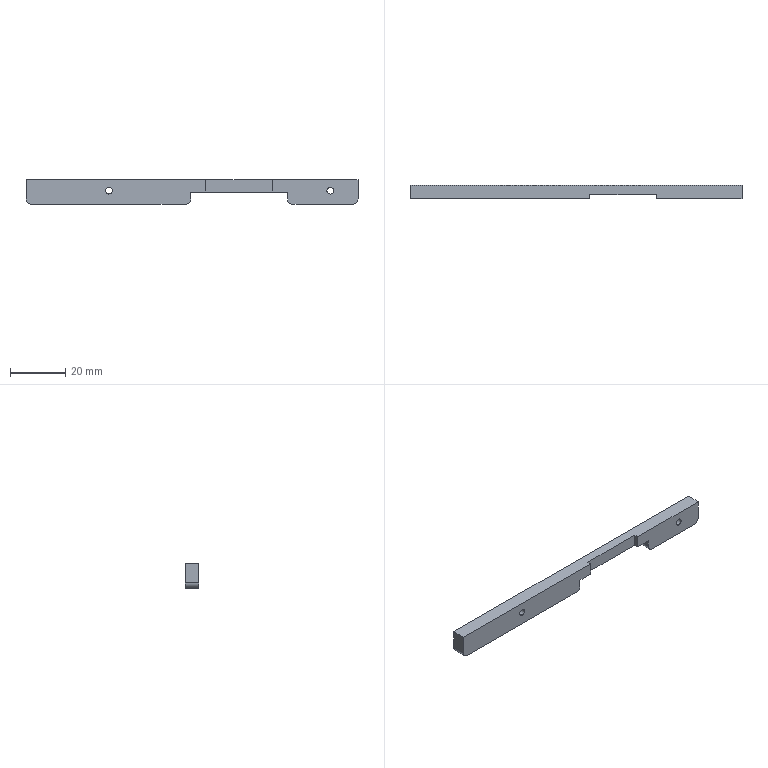Part | SolidWorks | features Fillet 2, ICE 2, Extrusion 1, HoleWzd 1 | 1 solid | 22 faces | box 120 x 5 x 9 mm | volume 4384 mm3 | plane 14 | cylinder 8 | commonest cylinder face diameters 2.5 x4 4 x4
STEP:
#1=CARTESIAN_POINT('',(30.,0.,-2.75));
#2=VERTEX_POINT('',#1);
#3=CARTESIAN_POINT('',(30.,0.,-5.25));
#4=VERTEX_POINT('',#3);
#5=CARTESIAN_POINT('',(30.,0.,-4.));
#6=DIRECTION('',(0.,-1.,0.));
#7=DIRECTION('',(0.,0.,-1.));
#8=AXIS2_PLACEMENT_3D('',#5,#6,#7);
#9=CIRCLE('',#8,1.25);
#10=EDGE_CURVE('',#2,#4,#9,.T.);
#11=ORIENTED_EDGE('',*,*,#10,.T.);
#12=CARTESIAN_POINT('',(30.,5.,-5.25));
#13=VERTEX_POINT('',#12);
#14=CARTESIAN_POINT('',(30.,5.,-5.25));
#15=DIRECTION('',(0.,1.,0.));
#16=VECTOR('',#15,1000.);
#17=LINE('',#14,#16);
#18=EDGE_CURVE('',#4,#13,#17,.T.);
#19=ORIENTED_EDGE('',*,*,#18,.T.);
#20=CARTESIAN_POINT('',(30.,5.,-2.75));
#21=VERTEX_POINT('',#20);
#22=CARTESIAN_POINT('',(30.,5.,-4.));
#23=DIRECTION('',(0.,1.,0.));
#24=DIRECTION('',(0.,0.,1.));
#25=AXIS2_PLACEMENT_3D('',#22,#23,#24);
#26=CIRCLE('',#25,1.25);
#27=EDGE_CURVE('',#13,#21,#26,.T.);
#28=ORIENTED_EDGE('',*,*,#27,.T.);
#29=CARTESIAN_POINT('',(30.,5.,-2.75));
#30=DIRECTION('',(0.,1.,0.));
#31=VECTOR('',#30,1000.);
#32=LINE('',#29,#31);
#33=EDGE_CURVE('',#2,#21,#32,.T.);
#34=ORIENTED_EDGE('',*,*,#33,.F.);
#35=EDGE_LOOP('',(#11,#19,#28,#34));
#36=FACE_OUTER_BOUND('',#35,.T.);
#37=CARTESIAN_POINT('',(30.,5.,-4.));
#38=DIRECTION('',(0.,1.,0.));
#39=DIRECTION('',(0.,0.,1.));
#40=AXIS2_PLACEMENT_3D('',#37,#38,#39);
#41=CYLINDRICAL_SURFACE('',#40,1.25);
#42=ADVANCED_FACE('',(#36),#41,.F.);
#43=CARTESIAN_POINT('',(110.,0.,-2.75));
#44=VERTEX_POINT('',#43);
#45=CARTESIAN_POINT('',(110.,0.,-5.25));
#46=VERTEX_POINT('',#45);
#47=CARTESIAN_POINT('',(110.,0.,-4.));
#48=DIRECTION('',(0.,-1.,0.));
#49=DIRECTION('',(0.,0.,-1.));
#50=AXIS2_PLACEMENT_3D('',#47,#48,#49);
#51=CIRCLE('',#50,1.25);
#52=EDGE_CURVE('',#44,#46,#51,.T.);
#53=ORIENTED_EDGE('',*,*,#52,.T.);
#54=CARTESIAN_POINT('',(110.,5.,-5.25));
#55=VERTEX_POINT('',#54);
#56=CARTESIAN_POINT('',(110.,5.,-5.25));
#57=DIRECTION('',(0.,1.,0.));
#58=VECTOR('',#57,1000.);
#59=LINE('',#56,#58);
#60=EDGE_CURVE('',#46,#55,#59,.T.);
#61=ORIENTED_EDGE('',*,*,#60,.T.);
#62=CARTESIAN_POINT('',(110.,5.,-2.75));
#63=VERTEX_POINT('',#62);
#64=CARTESIAN_POINT('',(110.,5.,-4.));
#65=DIRECTION('',(0.,1.,0.));
#66=DIRECTION('',(0.,0.,1.));
#67=AXIS2_PLACEMENT_3D('',#64,#65,#66);
#68=CIRCLE('',#67,1.25);
#69=EDGE_CURVE('',#55,#63,#68,.T.);
#70=ORIENTED_EDGE('',*,*,#69,.T.);
#71=CARTESIAN_POINT('',(110.,5.,-2.75));
#72=DIRECTION('',(0.,1.,0.));
#73=VECTOR('',#72,1000.);
#74=LINE('',#71,#73);
#75=EDGE_CURVE('',#44,#63,#74,.T.);
#76=ORIENTED_EDGE('',*,*,#75,.F.);
#77=EDGE_LOOP('',(#53,#61,#70,#76));
#78=FACE_OUTER_BOUND('',#77,.T.);
#79=CARTESIAN_POINT('',(110.,5.,-4.));
#80=DIRECTION('',(0.,1.,0.));
#81=DIRECTION('',(0.,0.,1.));
#82=AXIS2_PLACEMENT_3D('',#79,#80,#81);
#83=CYLINDRICAL_SURFACE('',#82,1.25);
#84=ADVANCED_FACE('',(#78),#83,.F.);
#85=CARTESIAN_POINT('',(65.,0.,0.));
#86=VERTEX_POINT('',#85);
#87=CARTESIAN_POINT('',(65.,0.,-4.5));
#88=VERTEX_POINT('',#87);
#89=CARTESIAN_POINT('',(65.,0.,-9.));
#90=DIRECTION('',(0.,0.,-1.));
#91=VECTOR('',#90,1000.);
#92=LINE('',#89,#91);
#93=EDGE_CURVE('',#86,#88,#92,.T.);
#94=ORIENTED_EDGE('',*,*,#93,.F.);
#95=CARTESIAN_POINT('',(0.,0.,0.));
#96=VERTEX_POINT('',#95);
#97=CARTESIAN_POINT('',(120.,0.,0.));
#98=DIRECTION('',(1.,0.,0.));
#99=VECTOR('',#98,1000.);
#100=LINE('',#97,#99);
#101=EDGE_CURVE('',#96,#86,#100,.T.);
#102=ORIENTED_EDGE('',*,*,#101,.F.);
#103=CARTESIAN_POINT('',(0.,0.,-7.));
#104=VERTEX_POINT('',#103);
#105=CARTESIAN_POINT('',(0.,0.,0.));
#106=DIRECTION('',(0.,0.,1.));
#107=VECTOR('',#106,1000.);
#108=LINE('',#105,#107);
#109=EDGE_CURVE('',#104,#96,#108,.T.);
#110=ORIENTED_EDGE('',*,*,#109,.F.);
#111=CARTESIAN_POINT('',(2.,0.,-9.));
#112=VERTEX_POINT('',#111);
#113=CARTESIAN_POINT('',(2.,0.,-7.));
#114=DIRECTION('',(0.,-1.,0.));
#115=DIRECTION('',(0.,0.,-1.));
#116=AXIS2_PLACEMENT_3D('',#113,#114,#115);
#117=CIRCLE('',#116,2.);
#118=EDGE_CURVE('',#104,#112,#117,.T.);
#119=ORIENTED_EDGE('',*,*,#118,.T.);
#120=CARTESIAN_POINT('',(57.5,0.,-9.));
#121=VERTEX_POINT('',#120);
#122=CARTESIAN_POINT('',(0.,0.,-9.));
#123=DIRECTION('',(-1.,0.,0.));
#124=VECTOR('',#123,1000.);
#125=LINE('',#122,#124);
#126=EDGE_CURVE('',#121,#112,#125,.T.);
#127=ORIENTED_EDGE('',*,*,#126,.F.);
#128=CARTESIAN_POINT('',(59.5,0.,-7.));
#129=VERTEX_POINT('',#128);
#130=CARTESIAN_POINT('',(57.5,0.,-7.));
#131=DIRECTION('',(0.,-1.,0.));
#132=DIRECTION('',(0.,0.,-1.));
#133=AXIS2_PLACEMENT_3D('',#130,#131,#132);
#134=CIRCLE('',#133,2.);
#135=EDGE_CURVE('',#121,#129,#134,.T.);
#136=ORIENTED_EDGE('',*,*,#135,.T.);
#137=CARTESIAN_POINT('',(59.5,0.,-4.5));
#138=VERTEX_POINT('',#137);
#139=CARTESIAN_POINT('',(59.5,0.,-9.));
#140=DIRECTION('',(0.,0.,1.));
#141=VECTOR('',#140,1000.);
#142=LINE('',#139,#141);
#143=EDGE_CURVE('',#129,#138,#142,.T.);
#144=ORIENTED_EDGE('',*,*,#143,.T.);
#145=CARTESIAN_POINT('',(94.5,0.,-4.5));
#146=DIRECTION('',(1.,0.,0.));
#147=VECTOR('',#146,1000.);
#148=LINE('',#145,#147);
#149=EDGE_CURVE('',#138,#88,#148,.T.);
#150=ORIENTED_EDGE('',*,*,#149,.T.);
#151=EDGE_LOOP('',(#94,#102,#110,#119,#127,#136,#144,#150));
#152=FACE_OUTER_BOUND('',#151,.T.);
#153=ORIENTED_EDGE('',*,*,#10,.F.);
#154=CARTESIAN_POINT('',(30.,0.,-4.));
#155=DIRECTION('',(0.,-1.,0.));
#156=DIRECTION('',(0.,0.,-1.));
#157=AXIS2_PLACEMENT_3D('',#154,#155,#156);
#158=CIRCLE('',#157,1.25);
#159=EDGE_CURVE('',#4,#2,#158,.T.);
#160=ORIENTED_EDGE('',*,*,#159,.F.);
#161=EDGE_LOOP('',(#153,#160));
#162=FACE_BOUND('',#161,.T.);
#163=CARTESIAN_POINT('',(0.,0.,0.));
#164=DIRECTION('',(0.,-1.,0.));
#165=DIRECTION('',(0.,0.,-1.));
#166=AXIS2_PLACEMENT_3D('',#163,#164,#165);
#167=PLANE('',#166);
#168=ADVANCED_FACE('',(#152,#162),#167,.T.);
#169=CARTESIAN_POINT('',(118.,0.,-9.));
#170=VERTEX_POINT('',#169);
#171=CARTESIAN_POINT('',(96.5,0.,-9.));
#172=VERTEX_POINT('',#171);
#173=CARTESIAN_POINT('',(0.,0.,-9.));
#174=DIRECTION('',(-1.,0.,0.));
#175=VECTOR('',#174,1000.);
#176=LINE('',#173,#175);
#177=EDGE_CURVE('',#170,#172,#176,.T.);
#178=ORIENTED_EDGE('',*,*,#177,.T.);
#179=CARTESIAN_POINT('',(96.5,5.,-9.));
#180=VERTEX_POINT('',#179);
#181=CARTESIAN_POINT('',(96.5,5.,-9.));
#182=DIRECTION('',(0.,1.,0.));
#183=VECTOR('',#182,1000.);
#184=LINE('',#181,#183);
#185=EDGE_CURVE('',#172,#180,#184,.T.);
#186=ORIENTED_EDGE('',*,*,#185,.T.);
#187=CARTESIAN_POINT('',(118.,5.,-9.));
#188=VERTEX_POINT('',#187);
#189=CARTESIAN_POINT('',(0.,5.,-9.));
#190=DIRECTION('',(-1.,0.,0.));
#191=VECTOR('',#190,1000.);
#192=LINE('',#189,#191);
#193=EDGE_CURVE('',#188,#180,#192,.T.);
#194=ORIENTED_EDGE('',*,*,#193,.F.);
#195=CARTESIAN_POINT('',(118.,5.,-9.));
#196=DIRECTION('',(0.,-1.,0.));
#197=VECTOR('',#196,1000.);
#198=LINE('',#195,#197);
#199=EDGE_CURVE('',#188,#170,#198,.T.);
#200=ORIENTED_EDGE('',*,*,#199,.T.);
#201=EDGE_LOOP('',(#178,#186,#194,#200));
#202=FACE_OUTER_BOUND('',#201,.T.);
#203=CARTESIAN_POINT('',(0.,5.,-9.));
#204=DIRECTION('',(0.,0.,1.));
#205=DIRECTION('',(1.,0.,0.));
#206=AXIS2_PLACEMENT_3D('',#203,#204,#205);
#207=PLANE('',#206);
#208=ADVANCED_FACE('',(#202),#207,.F.);
#209=ORIENTED_EDGE('',*,*,#101,.T.);
#210=CARTESIAN_POINT('',(65.,1.5,0.));
#211=VERTEX_POINT('',#210);
#212=CARTESIAN_POINT('',(65.,1.5,0.));
#213=DIRECTION('',(0.,-1.,0.));
#214=VECTOR('',#213,1000.);
#215=LINE('',#212,#214);
#216=EDGE_CURVE('',#211,#86,#215,.T.);
#217=ORIENTED_EDGE('',*,*,#216,.F.);
#218=CARTESIAN_POINT('',(89.,1.5,0.));
#219=VERTEX_POINT('',#218);
#220=CARTESIAN_POINT('',(89.,1.5,0.));
#221=DIRECTION('',(-1.,0.,0.));
#222=VECTOR('',#221,1000.);
#223=LINE('',#220,#222);
#224=EDGE_CURVE('',#219,#211,#223,.T.);
#225=ORIENTED_EDGE('',*,*,#224,.F.);
#226=CARTESIAN_POINT('',(89.,0.,0.));
#227=VERTEX_POINT('',#226);
#228=CARTESIAN_POINT('',(89.,1.5,0.));
#229=DIRECTION('',(0.,-1.,0.));
#230=VECTOR('',#229,1000.);
#231=LINE('',#228,#230);
#232=EDGE_CURVE('',#219,#227,#231,.T.);
#233=ORIENTED_EDGE('',*,*,#232,.T.);
#234=CARTESIAN_POINT('',(120.,0.,0.));
#235=VERTEX_POINT('',#234);
#236=CARTESIAN_POINT('',(120.,0.,0.));
#237=DIRECTION('',(1.,0.,0.));
#238=VECTOR('',#237,1000.);
#239=LINE('',#236,#238);
#240=EDGE_CURVE('',#227,#235,#239,.T.);
#241=ORIENTED_EDGE('',*,*,#240,.T.);
#242=CARTESIAN_POINT('',(120.,5.,0.));
#243=VERTEX_POINT('',#242);
#244=CARTESIAN_POINT('',(120.,5.,0.));
#245=DIRECTION('',(0.,-1.,0.));
#246=VECTOR('',#245,1000.);
#247=LINE('',#244,#246);
#248=EDGE_CURVE('',#243,#235,#247,.T.);
#249=ORIENTED_EDGE('',*,*,#248,.F.);
#250=CARTESIAN_POINT('',(0.,5.,0.));
#251=VERTEX_POINT('',#250);
#252=CARTESIAN_POINT('',(120.,5.,0.));
#253=DIRECTION('',(1.,0.,0.));
#254=VECTOR('',#253,1000.);
#255=LINE('',#252,#254);
#256=EDGE_CURVE('',#251,#243,#255,.T.);
#257=ORIENTED_EDGE('',*,*,#256,.F.);
#258=CARTESIAN_POINT('',(0.,5.,0.));
#259=DIRECTION('',(0.,-1.,0.));
#260=VECTOR('',#259,1000.);
#261=LINE('',#258,#260);
#262=EDGE_CURVE('',#251,#96,#261,.T.);
#263=ORIENTED_EDGE('',*,*,#262,.T.);
#264=EDGE_LOOP('',(#209,#217,#225,#233,#241,#249,#257,#263));
#265=FACE_OUTER_BOUND('',#264,.T.);
#266=CARTESIAN_POINT('',(120.,5.,0.));
#267=DIRECTION('',(0.,0.,-1.));
#268=DIRECTION('',(-1.,0.,0.));
#269=AXIS2_PLACEMENT_3D('',#266,#267,#268);
#270=PLANE('',#269);
#271=ADVANCED_FACE('',(#265),#270,.F.);
#272=CARTESIAN_POINT('',(120.,0.,-7.));
#273=VERTEX_POINT('',#272);
#274=CARTESIAN_POINT('',(120.,0.,-9.));
#275=DIRECTION('',(0.,0.,-1.));
#276=VECTOR('',#275,1000.);
#277=LINE('',#274,#276);
#278=EDGE_CURVE('',#235,#273,#277,.T.);
#279=ORIENTED_EDGE('',*,*,#278,.T.);
#280=CARTESIAN_POINT('',(120.,5.,-7.));
#281=VERTEX_POINT('',#280);
#282=CARTESIAN_POINT('',(120.,5.,-7.));
#283=DIRECTION('',(0.,1.,0.));
#284=VECTOR('',#283,1000.);
#285=LINE('',#282,#284);
#286=EDGE_CURVE('',#273,#281,#285,.T.);
#287=ORIENTED_EDGE('',*,*,#286,.T.);
#288=CARTESIAN_POINT('',(120.,5.,-9.));
#289=DIRECTION('',(0.,0.,-1.));
#290=VECTOR('',#289,1000.);
#291=LINE('',#288,#290);
#292=EDGE_CURVE('',#243,#281,#291,.T.);
#293=ORIENTED_EDGE('',*,*,#292,.F.);
#294=ORIENTED_EDGE('',*,*,#248,.T.);
#295=EDGE_LOOP('',(#279,#287,#293,#294));
#296=FACE_OUTER_BOUND('',#295,.T.);
#297=CARTESIAN_POINT('',(120.,5.,-9.));
#298=DIRECTION('',(-1.,0.,0.));
#299=DIRECTION('',(0.,0.,1.));
#300=AXIS2_PLACEMENT_3D('',#297,#298,#299);
#301=PLANE('',#300);
#302=ADVANCED_FACE('',(#296),#301,.F.);
#303=CARTESIAN_POINT('',(57.5,5.,-9.));
#304=VERTEX_POINT('',#303);
#305=CARTESIAN_POINT('',(2.,5.,-9.));
#306=VERTEX_POINT('',#305);
#307=CARTESIAN_POINT('',(0.,5.,-9.));
#308=DIRECTION('',(-1.,0.,0.));
#309=VECTOR('',#308,1000.);
#310=LINE('',#307,#309);
#311=EDGE_CURVE('',#304,#306,#310,.T.);
#312=ORIENTED_EDGE('',*,*,#311,.F.);
#313=CARTESIAN_POINT('',(57.5,5.,-9.));
#314=DIRECTION('',(0.,-1.,0.));
#315=VECTOR('',#314,1000.);
#316=LINE('',#313,#315);
#317=EDGE_CURVE('',#304,#121,#316,.T.);
#318=ORIENTED_EDGE('',*,*,#317,.T.);
#319=ORIENTED_EDGE('',*,*,#126,.T.);
#320=CARTESIAN_POINT('',(2.,5.,-9.));
#321=DIRECTION('',(0.,1.,0.));
#322=VECTOR('',#321,1000.);
#323=LINE('',#320,#322);
#324=EDGE_CURVE('',#112,#306,#323,.T.);
#325=ORIENTED_EDGE('',*,*,#324,.T.);
#326=EDGE_LOOP('',(#312,#318,#319,#325));
#327=FACE_OUTER_BOUND('',#326,.T.);
#328=CARTESIAN_POINT('',(0.,5.,-9.));
#329=DIRECTION('',(0.,0.,1.));
#330=DIRECTION('',(1.,0.,0.));
#331=AXIS2_PLACEMENT_3D('',#328,#329,#330);
#332=PLANE('',#331);
#333=ADVANCED_FACE('',(#327),#332,.F.);
#334=CARTESIAN_POINT('',(0.,5.,-7.));
#335=VERTEX_POINT('',#334);
#336=CARTESIAN_POINT('',(0.,5.,0.));
#337=DIRECTION('',(0.,0.,1.));
#338=VECTOR('',#337,1000.);
#339=LINE('',#336,#338);
#340=EDGE_CURVE('',#335,#251,#339,.T.);
#341=ORIENTED_EDGE('',*,*,#340,.F.);
#342=CARTESIAN_POINT('',(0.,5.,-7.));
#343=DIRECTION('',(0.,-1.,0.));
#344=VECTOR('',#343,1000.);
#345=LINE('',#342,#344);
#346=EDGE_CURVE('',#335,#104,#345,.T.);
#347=ORIENTED_EDGE('',*,*,#346,.T.);
#348=ORIENTED_EDGE('',*,*,#109,.T.);
#349=ORIENTED_EDGE('',*,*,#262,.F.);
#350=EDGE_LOOP('',(#341,#347,#348,#349));
#351=FACE_OUTER_BOUND('',#350,.T.);
#352=CARTESIAN_POINT('',(0.,5.,0.));
#353=DIRECTION('',(1.,0.,0.));
#354=DIRECTION('',(0.,0.,-1.));
#355=AXIS2_PLACEMENT_3D('',#352,#353,#354);
#356=PLANE('',#355);
#357=ADVANCED_FACE('',(#351),#356,.F.);
#358=CARTESIAN_POINT('',(30.,5.,-4.));
#359=DIRECTION('',(0.,1.,0.));
#360=DIRECTION('',(0.,0.,1.));
#361=AXIS2_PLACEMENT_3D('',#358,#359,#360);
#362=CIRCLE('',#361,1.25);
#363=EDGE_CURVE('',#21,#13,#362,.T.);
#364=ORIENTED_EDGE('',*,*,#363,.F.);
#365=ORIENTED_EDGE('',*,*,#27,.F.);
#366=EDGE_LOOP('',(#364,#365));
#367=FACE_BOUND('',#366,.T.);
#368=CARTESIAN_POINT('',(110.,5.,-4.));
#369=DIRECTION('',(0.,1.,0.));
#370=DIRECTION('',(0.,0.,1.));
#371=AXIS2_PLACEMENT_3D('',#368,#369,#370);
#372=CIRCLE('',#371,1.25);
#373=EDGE_CURVE('',#63,#55,#372,.T.);
#374=ORIENTED_EDGE('',*,*,#373,.F.);
#375=ORIENTED_EDGE('',*,*,#69,.F.);
#376=EDGE_LOOP('',(#374,#375));
#377=FACE_BOUND('',#376,.T.);
#378=ORIENTED_EDGE('',*,*,#193,.T.);
#379=CARTESIAN_POINT('',(94.5,5.,-7.));
#380=VERTEX_POINT('',#379);
#381=CARTESIAN_POINT('',(96.5,5.,-7.));
#382=DIRECTION('',(0.,1.,0.));
#383=DIRECTION('',(0.,0.,-1.));
#384=AXIS2_PLACEMENT_3D('',#381,#382,#383);
#385=CIRCLE('',#384,2.);
#386=EDGE_CURVE('',#180,#380,#385,.T.);
#387=ORIENTED_EDGE('',*,*,#386,.T.);
#388=CARTESIAN_POINT('',(94.5,5.,-4.5));
#389=VERTEX_POINT('',#388);
#390=CARTESIAN_POINT('',(94.5,5.,-9.));
#391=DIRECTION('',(0.,0.,-1.));
#392=VECTOR('',#391,1000.);
#393=LINE('',#390,#392);
#394=EDGE_CURVE('',#389,#380,#393,.T.);
#395=ORIENTED_EDGE('',*,*,#394,.F.);
#396=CARTESIAN_POINT('',(59.5,5.,-4.5));
#397=VERTEX_POINT('',#396);
#398=CARTESIAN_POINT('',(94.5,5.,-4.5));
#399=DIRECTION('',(1.,0.,0.));
#400=VECTOR('',#399,1000.);
#401=LINE('',#398,#400);
#402=EDGE_CURVE('',#397,#389,#401,.T.);
#403=ORIENTED_EDGE('',*,*,#402,.F.);
#404=CARTESIAN_POINT('',(59.5,5.,-7.));
#405=VERTEX_POINT('',#404);
#406=CARTESIAN_POINT('',(59.5,5.,-9.));
#407=DIRECTION('',(0.,0.,1.));
#408=VECTOR('',#407,1000.);
#409=LINE('',#406,#408);
#410=EDGE_CURVE('',#405,#397,#409,.T.);
#411=ORIENTED_EDGE('',*,*,#410,.F.);
#412=CARTESIAN_POINT('',(57.5,5.,-7.));
#413=DIRECTION('',(0.,1.,0.));
#414=DIRECTION('',(0.,0.,-1.));
#415=AXIS2_PLACEMENT_3D('',#412,#413,#414);
#416=CIRCLE('',#415,2.);
#417=EDGE_CURVE('',#405,#304,#416,.T.);
#418=ORIENTED_EDGE('',*,*,#417,.T.);
#419=ORIENTED_EDGE('',*,*,#311,.T.);
#420=CARTESIAN_POINT('',(2.,5.,-7.));
#421=DIRECTION('',(0.,1.,0.));
#422=DIRECTION('',(0.,0.,-1.));
#423=AXIS2_PLACEMENT_3D('',#420,#421,#422);
#424=CIRCLE('',#423,2.);
#425=EDGE_CURVE('',#306,#335,#424,.T.);
#426=ORIENTED_EDGE('',*,*,#425,.T.);
#427=ORIENTED_EDGE('',*,*,#340,.T.);
#428=ORIENTED_EDGE('',*,*,#256,.T.);
#429=ORIENTED_EDGE('',*,*,#292,.T.);
#430=CARTESIAN_POINT('',(118.,5.,-7.));
#431=DIRECTION('',(0.,1.,0.));
#432=DIRECTION('',(0.,0.,-1.));
#433=AXIS2_PLACEMENT_3D('',#430,#431,#432);
#434=CIRCLE('',#433,2.);
#435=EDGE_CURVE('',#281,#188,#434,.T.);
#436=ORIENTED_EDGE('',*,*,#435,.T.);
#437=EDGE_LOOP('',(#378,#387,#395,#403,#411,#418,#419,#426,#427,#428,#429,#436));
#438=FACE_OUTER_BOUND('',#437,.T.);
#439=CARTESIAN_POINT('',(0.,5.,0.));
#440=DIRECTION('',(0.,-1.,0.));
#441=DIRECTION('',(0.,0.,-1.));
#442=AXIS2_PLACEMENT_3D('',#439,#440,#441);
#443=PLANE('',#442);
#444=ADVANCED_FACE('',(#367,#377,#438),#443,.F.);
#445=CARTESIAN_POINT('',(89.,0.,-4.5));
#446=VERTEX_POINT('',#445);
#447=CARTESIAN_POINT('',(89.,0.,-9.));
#448=DIRECTION('',(0.,0.,1.));
#449=VECTOR('',#448,1000.);
#450=LINE('',#447,#449);
#451=EDGE_CURVE('',#446,#227,#450,.T.);
#452=ORIENTED_EDGE('',*,*,#451,.F.);
#453=CARTESIAN_POINT('',(94.5,0.,-4.5));
#454=VERTEX_POINT('',#453);
#455=CARTESIAN_POINT('',(94.5,0.,-4.5));
#456=DIRECTION('',(1.,0.,0.));
#457=VECTOR('',#456,1000.);
#458=LINE('',#455,#457);
#459=EDGE_CURVE('',#446,#454,#458,.T.);
#460=ORIENTED_EDGE('',*,*,#459,.T.);
#461=CARTESIAN_POINT('',(94.5,0.,-7.));
#462=VERTEX_POINT('',#461);
#463=CARTESIAN_POINT('',(94.5,0.,-9.));
#464=DIRECTION('',(0.,0.,-1.));
#465=VECTOR('',#464,1000.);
#466=LINE('',#463,#465);
#467=EDGE_CURVE('',#454,#462,#466,.T.);
#468=ORIENTED_EDGE('',*,*,#467,.T.);
#469=CARTESIAN_POINT('',(96.5,0.,-7.));
#470=DIRECTION('',(0.,-1.,0.));
#471=DIRECTION('',(0.,0.,-1.));
#472=AXIS2_PLACEMENT_3D('',#469,#470,#471);
#473=CIRCLE('',#472,2.);
#474=EDGE_CURVE('',#462,#172,#473,.T.);
#475=ORIENTED_EDGE('',*,*,#474,.T.);
#476=ORIENTED_EDGE('',*,*,#177,.F.);
#477=CARTESIAN_POINT('',(118.,0.,-7.));
#478=DIRECTION('',(0.,-1.,0.));
#479=DIRECTION('',(0.,0.,-1.));
#480=AXIS2_PLACEMENT_3D('',#477,#478,#479);
#481=CIRCLE('',#480,2.);
#482=EDGE_CURVE('',#170,#273,#481,.T.);
#483=ORIENTED_EDGE('',*,*,#482,.T.);
#484=ORIENTED_EDGE('',*,*,#278,.F.);
#485=ORIENTED_EDGE('',*,*,#240,.F.);
#486=EDGE_LOOP('',(#452,#460,#468,#475,#476,#483,#484,#485));
#487=FACE_OUTER_BOUND('',#486,.T.);
#488=ORIENTED_EDGE('',*,*,#52,.F.);
#489=CARTESIAN_POINT('',(110.,0.,-4.));
#490=DIRECTION('',(0.,-1.,0.));
#491=DIRECTION('',(0.,0.,-1.));
#492=AXIS2_PLACEMENT_3D('',#489,#490,#491);
#493=CIRCLE('',#492,1.25);
#494=EDGE_CURVE('',#46,#44,#493,.T.);
#495=ORIENTED_EDGE('',*,*,#494,.F.);
#496=EDGE_LOOP('',(#488,#495));
#497=FACE_BOUND('',#496,.T.);
#498=CARTESIAN_POINT('',(0.,0.,0.));
#499=DIRECTION('',(0.,-1.,0.));
#500=DIRECTION('',(0.,0.,-1.));
#501=AXIS2_PLACEMENT_3D('',#498,#499,#500);
#502=PLANE('',#501);
#503=ADVANCED_FACE('',(#487,#497),#502,.T.);
#504=ORIENTED_EDGE('',*,*,#60,.F.);
#505=ORIENTED_EDGE('',*,*,#494,.T.);
#506=ORIENTED_EDGE('',*,*,#75,.T.);
#507=ORIENTED_EDGE('',*,*,#373,.T.);
#508=EDGE_LOOP('',(#504,#505,#506,#507));
#509=FACE_OUTER_BOUND('',#508,.T.);
#510=CARTESIAN_POINT('',(110.,5.,-4.));
#511=DIRECTION('',(0.,1.,0.));
#512=DIRECTION('',(0.,0.,1.));
#513=AXIS2_PLACEMENT_3D('',#510,#511,#512);
#514=CYLINDRICAL_SURFACE('',#513,1.25);
#515=ADVANCED_FACE('',(#509),#514,.F.);
#516=ORIENTED_EDGE('',*,*,#18,.F.);
#517=ORIENTED_EDGE('',*,*,#159,.T.);
#518=ORIENTED_EDGE('',*,*,#33,.T.);
#519=ORIENTED_EDGE('',*,*,#363,.T.);
#520=EDGE_LOOP('',(#516,#517,#518,#519));
#521=FACE_OUTER_BOUND('',#520,.T.);
#522=CARTESIAN_POINT('',(30.,5.,-4.));
#523=DIRECTION('',(0.,1.,0.));
#524=DIRECTION('',(0.,0.,1.));
#525=AXIS2_PLACEMENT_3D('',#522,#523,#524);
#526=CYLINDRICAL_SURFACE('',#525,1.25);
#527=ADVANCED_FACE('',(#521),#526,.F.);
#528=ORIENTED_EDGE('',*,*,#425,.F.);
#529=ORIENTED_EDGE('',*,*,#324,.F.);
#530=ORIENTED_EDGE('',*,*,#118,.F.);
#531=ORIENTED_EDGE('',*,*,#346,.F.);
#532=EDGE_LOOP('',(#528,#529,#530,#531));
#533=FACE_OUTER_BOUND('',#532,.T.);
#534=CARTESIAN_POINT('',(2.,5.,-7.));
#535=DIRECTION('',(0.,-1.,0.));
#536=DIRECTION('',(0.,0.,-1.));
#537=AXIS2_PLACEMENT_3D('',#534,#535,#536);
#538=CYLINDRICAL_SURFACE('',#537,2.);
#539=ADVANCED_FACE('',(#533),#538,.T.);
#540=ORIENTED_EDGE('',*,*,#435,.F.);
#541=ORIENTED_EDGE('',*,*,#286,.F.);
#542=ORIENTED_EDGE('',*,*,#482,.F.);
#543=ORIENTED_EDGE('',*,*,#199,.F.);
#544=EDGE_LOOP('',(#540,#541,#542,#543));
#545=FACE_OUTER_BOUND('',#544,.T.);
#546=CARTESIAN_POINT('',(118.,5.,-7.));
#547=DIRECTION('',(0.,-1.,0.));
#548=DIRECTION('',(0.,0.,-1.));
#549=AXIS2_PLACEMENT_3D('',#546,#547,#548);
#550=CYLINDRICAL_SURFACE('',#549,2.);
#551=ADVANCED_FACE('',(#545),#550,.T.);
#552=ORIENTED_EDGE('',*,*,#394,.T.);
#553=CARTESIAN_POINT('',(94.5,0.,-7.));
#554=DIRECTION('',(0.,-1.,0.));
#555=VECTOR('',#554,1000.);
#556=LINE('',#553,#555);
#557=EDGE_CURVE('',#380,#462,#556,.T.);
#558=ORIENTED_EDGE('',*,*,#557,.T.);
#559=ORIENTED_EDGE('',*,*,#467,.F.);
#560=CARTESIAN_POINT('',(94.5,0.,-4.5));
#561=DIRECTION('',(0.,1.,0.));
#562=VECTOR('',#561,1000.);
#563=LINE('',#560,#562);
#564=EDGE_CURVE('',#454,#389,#563,.T.);
#565=ORIENTED_EDGE('',*,*,#564,.T.);
#566=EDGE_LOOP('',(#552,#558,#559,#565));
#567=FACE_OUTER_BOUND('',#566,.T.);
#568=CARTESIAN_POINT('',(94.5,0.,-9.));
#569=DIRECTION('',(1.,0.,0.));
#570=DIRECTION('',(0.,0.,-1.));
#571=AXIS2_PLACEMENT_3D('',#568,#569,#570);
#572=PLANE('',#571);
#573=ADVANCED_FACE('',(#567),#572,.F.);
#574=CARTESIAN_POINT('',(65.,1.5,-4.5));
#575=VERTEX_POINT('',#574);
#576=CARTESIAN_POINT('',(89.,1.5,-4.5));
#577=VERTEX_POINT('',#576);
#578=CARTESIAN_POINT('',(94.5,1.5,-4.5));
#579=DIRECTION('',(1.,0.,0.));
#580=VECTOR('',#579,1000.);
#581=LINE('',#578,#580);
#582=EDGE_CURVE('',#575,#577,#581,.T.);
#583=ORIENTED_EDGE('',*,*,#582,.F.);
#584=CARTESIAN_POINT('',(65.,0.,-4.5));
#585=DIRECTION('',(0.,-1.,0.));
#586=VECTOR('',#585,1000.);
#587=LINE('',#584,#586);
#588=EDGE_CURVE('',#575,#88,#587,.T.);
#589=ORIENTED_EDGE('',*,*,#588,.T.);
#590=ORIENTED_EDGE('',*,*,#149,.F.);
#591=CARTESIAN_POINT('',(59.5,0.,-4.5));
#592=DIRECTION('',(0.,1.,0.));
#593=VECTOR('',#592,1000.);
#594=LINE('',#591,#593);
#595=EDGE_CURVE('',#138,#397,#594,.T.);
#596=ORIENTED_EDGE('',*,*,#595,.T.);
#597=ORIENTED_EDGE('',*,*,#402,.T.);
#598=ORIENTED_EDGE('',*,*,#564,.F.);
#599=ORIENTED_EDGE('',*,*,#459,.F.);
#600=CARTESIAN_POINT('',(89.,0.,-4.5));
#601=DIRECTION('',(0.,1.,0.));
#602=VECTOR('',#601,1000.);
#603=LINE('',#600,#602);
#604=EDGE_CURVE('',#446,#577,#603,.T.);
#605=ORIENTED_EDGE('',*,*,#604,.T.);
#606=EDGE_LOOP('',(#583,#589,#590,#596,#597,#598,#599,#605));
#607=FACE_OUTER_BOUND('',#606,.T.);
#608=CARTESIAN_POINT('',(94.5,0.,-4.5));
#609=DIRECTION('',(0.,0.,1.));
#610=DIRECTION('',(1.,0.,0.));
#611=AXIS2_PLACEMENT_3D('',#608,#609,#610);
#612=PLANE('',#611);
#613=ADVANCED_FACE('',(#607),#612,.F.);
#614=ORIENTED_EDGE('',*,*,#143,.F.);
#615=CARTESIAN_POINT('',(59.5,0.,-7.));
#616=DIRECTION('',(0.,1.,0.));
#617=VECTOR('',#616,1000.);
#618=LINE('',#615,#617);
#619=EDGE_CURVE('',#129,#405,#618,.T.);
#620=ORIENTED_EDGE('',*,*,#619,.T.);
#621=ORIENTED_EDGE('',*,*,#410,.T.);
#622=ORIENTED_EDGE('',*,*,#595,.F.);
#623=EDGE_LOOP('',(#614,#620,#621,#622));
#624=FACE_OUTER_BOUND('',#623,.T.);
#625=CARTESIAN_POINT('',(59.5,0.,-9.));
#626=DIRECTION('',(-1.,0.,0.));
#627=DIRECTION('',(0.,0.,1.));
#628=AXIS2_PLACEMENT_3D('',#625,#626,#627);
#629=PLANE('',#628);
#630=ADVANCED_FACE('',(#624),#629,.F.);
#631=ORIENTED_EDGE('',*,*,#474,.F.);
#632=ORIENTED_EDGE('',*,*,#557,.F.);
#633=ORIENTED_EDGE('',*,*,#386,.F.);
#634=ORIENTED_EDGE('',*,*,#185,.F.);
#635=EDGE_LOOP('',(#631,#632,#633,#634));
#636=FACE_OUTER_BOUND('',#635,.T.);
#637=CARTESIAN_POINT('',(96.5,5.,-7.));
#638=DIRECTION('',(0.,1.,0.));
#639=DIRECTION('',(0.,0.,1.));
#640=AXIS2_PLACEMENT_3D('',#637,#638,#639);
#641=CYLINDRICAL_SURFACE('',#640,2.);
#642=ADVANCED_FACE('',(#636),#641,.T.);
#643=ORIENTED_EDGE('',*,*,#135,.F.);
#644=ORIENTED_EDGE('',*,*,#317,.F.);
#645=ORIENTED_EDGE('',*,*,#417,.F.);
#646=ORIENTED_EDGE('',*,*,#619,.F.);
#647=EDGE_LOOP('',(#643,#644,#645,#646));
#648=FACE_OUTER_BOUND('',#647,.T.);
#649=CARTESIAN_POINT('',(57.5,0.,-7.));
#650=DIRECTION('',(0.,1.,0.));
#651=DIRECTION('',(0.,0.,1.));
#652=AXIS2_PLACEMENT_3D('',#649,#650,#651);
#653=CYLINDRICAL_SURFACE('',#652,2.);
#654=ADVANCED_FACE('',(#648),#653,.T.);
#655=CARTESIAN_POINT('',(65.,1.5,-9.));
#656=DIRECTION('',(0.,0.,-1.));
#657=VECTOR('',#656,1000.);
#658=LINE('',#655,#657);
#659=EDGE_CURVE('',#211,#575,#658,.T.);
#660=ORIENTED_EDGE('',*,*,#659,.F.);
#661=ORIENTED_EDGE('',*,*,#216,.T.);
#662=ORIENTED_EDGE('',*,*,#93,.T.);
#663=ORIENTED_EDGE('',*,*,#588,.F.);
#664=EDGE_LOOP('',(#660,#661,#662,#663));
#665=FACE_OUTER_BOUND('',#664,.T.);
#666=CARTESIAN_POINT('',(65.,1.5,-9.));
#667=DIRECTION('',(-1.,0.,0.));
#668=DIRECTION('',(0.,0.,1.));
#669=AXIS2_PLACEMENT_3D('',#666,#667,#668);
#670=PLANE('',#669);
#671=ADVANCED_FACE('',(#665),#670,.F.);
#672=ORIENTED_EDGE('',*,*,#451,.T.);
#673=ORIENTED_EDGE('',*,*,#232,.F.);
#674=CARTESIAN_POINT('',(89.,1.5,-9.));
#675=DIRECTION('',(0.,0.,1.));
#676=VECTOR('',#675,1000.);
#677=LINE('',#674,#676);
#678=EDGE_CURVE('',#577,#219,#677,.T.);
#679=ORIENTED_EDGE('',*,*,#678,.F.);
#680=ORIENTED_EDGE('',*,*,#604,.F.);
#681=EDGE_LOOP('',(#672,#673,#679,#680));
#682=FACE_OUTER_BOUND('',#681,.T.);
#683=CARTESIAN_POINT('',(89.,1.5,-9.));
#684=DIRECTION('',(1.,0.,0.));
#685=DIRECTION('',(0.,0.,-1.));
#686=AXIS2_PLACEMENT_3D('',#683,#684,#685);
#687=PLANE('',#686);
#688=ADVANCED_FACE('',(#682),#687,.F.);
#689=ORIENTED_EDGE('',*,*,#582,.T.);
#690=ORIENTED_EDGE('',*,*,#678,.T.);
#691=ORIENTED_EDGE('',*,*,#224,.T.);
#692=ORIENTED_EDGE('',*,*,#659,.T.);
#693=EDGE_LOOP('',(#689,#690,#691,#692));
#694=FACE_OUTER_BOUND('',#693,.T.);
#695=CARTESIAN_POINT('',(0.,1.5,0.));
#696=DIRECTION('',(0.,-1.,0.));
#697=DIRECTION('',(0.,0.,-1.));
#698=AXIS2_PLACEMENT_3D('',#695,#696,#697);
#699=PLANE('',#698);
#700=ADVANCED_FACE('',(#694),#699,.T.);
#701=CLOSED_SHELL('',(#42,#84,#168,#208,#271,#302,#333,#357,#444,#503,#515,#527,#539,#551,#573,#613,#630,#642,#654,#671,#688,#700));
#702=MANIFOLD_SOLID_BREP('',#701);
#703=CARTESIAN_POINT('',(0.,0.,0.));
#704=DIRECTION('',(0.,0.,1.));
#705=DIRECTION('',(1.,0.,0.));
#706=AXIS2_PLACEMENT_3D('',#703,#704,#705);
#707=(LENGTH_UNIT()NAMED_UNIT(*)SI_UNIT(.MILLI.,.METRE.));
#708=UNCERTAINTY_MEASURE_WITH_UNIT(LENGTH_MEASURE(0.00001),#707,'','');
#709=(NAMED_UNIT(*)PLANE_ANGLE_UNIT()SI_UNIT($,.RADIAN.));
#710=(NAMED_UNIT(*)SI_UNIT($,.STERADIAN.)SOLID_ANGLE_UNIT());
#711=(GEOMETRIC_REPRESENTATION_CONTEXT(3)GLOBAL_UNCERTAINTY_ASSIGNED_CONTEXT((#708))GLOBAL_UNIT_ASSIGNED_CONTEXT((#707,#709,#710))REPRESENTATION_CONTEXT('',''));
#712=ADVANCED_BREP_SHAPE_REPRESENTATION('',(#702,#706),#711);